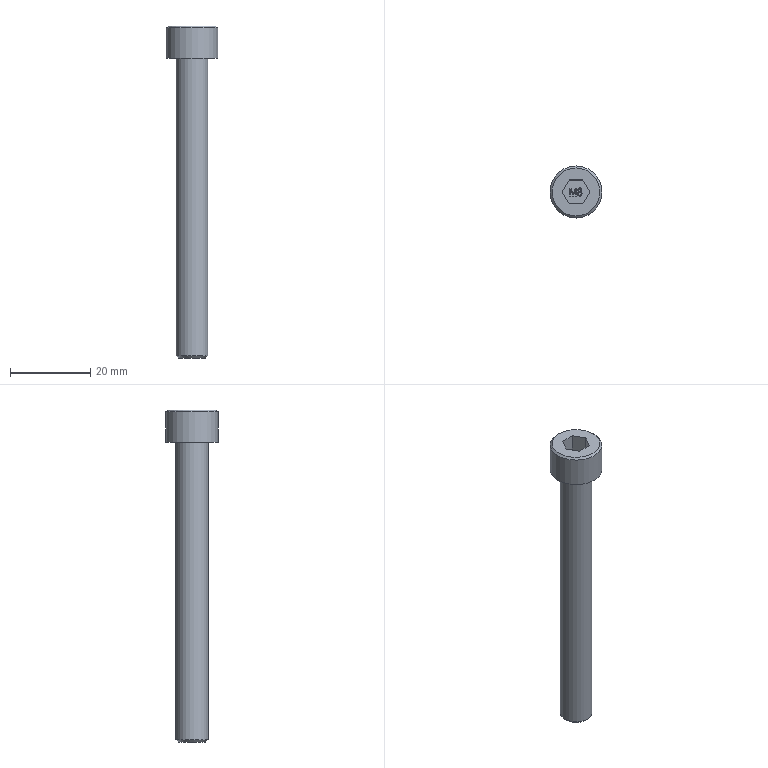Part | STEP file | EM10807500 | 1 solid | 38 faces | box 13 x 13 x 83 mm | volume 4667 mm3 | plane 25 | other 9 | cone 2 | cylinder 2 | commonest cylinder face diameters 8 x1 13 x1